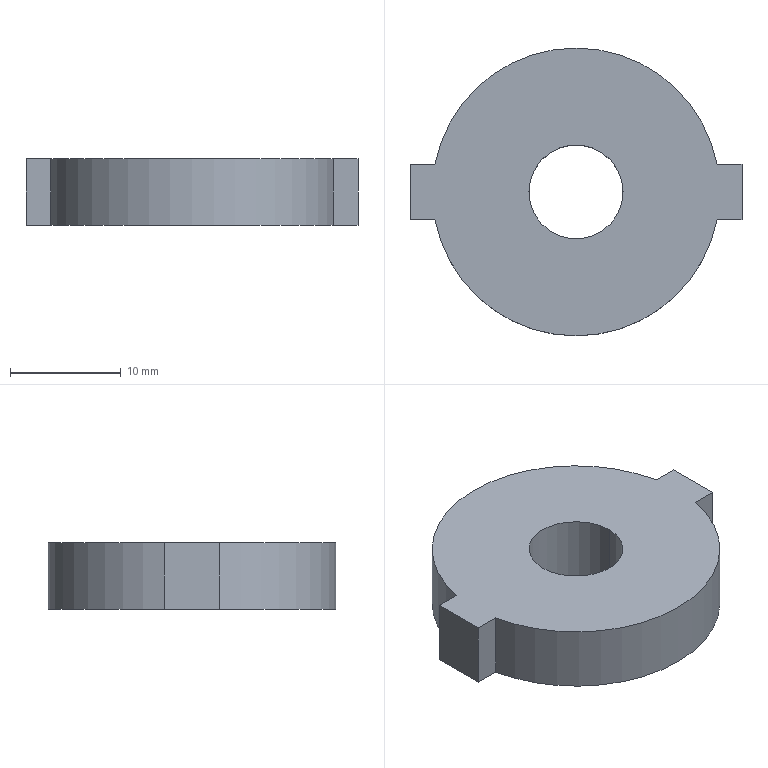Part | SolidWorks | features Extrusion 1 | 1 solid | 12 faces | box 30 x 26 x 6 mm | volume 2970 mm3 | plane 8 | cylinder 4 | commonest cylinder face diameters 8.5 x2 26 x2
STEP:
#1=CARTESIAN_POINT('',(-4.25,0.,0.));
#2=VERTEX_POINT('',#1);
#3=CARTESIAN_POINT('',(4.25,0.,0.));
#4=VERTEX_POINT('',#3);
#5=CARTESIAN_POINT('',(0.,0.,0.));
#6=DIRECTION('',(0.,0.,1.));
#7=DIRECTION('',(-1.,0.,0.));
#8=AXIS2_PLACEMENT_3D('',#5,#6,#7);
#9=CIRCLE('',#8,4.25);
#10=EDGE_CURVE('',#2,#4,#9,.T.);
#11=ORIENTED_EDGE('',*,*,#10,.F.);
#12=CARTESIAN_POINT('',(-4.25,0.,6.));
#13=VERTEX_POINT('',#12);
#14=CARTESIAN_POINT('',(-4.25,0.,0.));
#15=DIRECTION('',(0.,0.,1.));
#16=VECTOR('',#15,1000.);
#17=LINE('',#14,#16);
#18=EDGE_CURVE('',#2,#13,#17,.T.);
#19=ORIENTED_EDGE('',*,*,#18,.T.);
#20=CARTESIAN_POINT('',(4.25,0.,6.));
#21=VERTEX_POINT('',#20);
#22=CARTESIAN_POINT('',(0.,0.,6.));
#23=DIRECTION('',(0.,0.,1.));
#24=DIRECTION('',(-1.,0.,0.));
#25=AXIS2_PLACEMENT_3D('',#22,#23,#24);
#26=CIRCLE('',#25,4.25);
#27=EDGE_CURVE('',#13,#21,#26,.T.);
#28=ORIENTED_EDGE('',*,*,#27,.T.);
#29=CARTESIAN_POINT('',(4.25,0.,0.));
#30=DIRECTION('',(0.,0.,1.));
#31=VECTOR('',#30,1000.);
#32=LINE('',#29,#31);
#33=EDGE_CURVE('',#4,#21,#32,.T.);
#34=ORIENTED_EDGE('',*,*,#33,.F.);
#35=EDGE_LOOP('',(#11,#19,#28,#34));
#36=FACE_OUTER_BOUND('',#35,.T.);
#37=CARTESIAN_POINT('',(0.,0.,0.));
#38=DIRECTION('',(0.,0.,1.));
#39=DIRECTION('',(1.,0.,0.));
#40=AXIS2_PLACEMENT_3D('',#37,#38,#39);
#41=CYLINDRICAL_SURFACE('',#40,4.25);
#42=ADVANCED_FACE('',(#36),#41,.F.);
#43=CARTESIAN_POINT('',(12.757,2.5,6.));
#44=VERTEX_POINT('',#43);
#45=CARTESIAN_POINT('',(-12.757,2.5,6.));
#46=VERTEX_POINT('',#45);
#47=CARTESIAN_POINT('',(0.,0.,6.));
#48=DIRECTION('',(0.,0.,1.));
#49=DIRECTION('',(1.,0.,0.));
#50=AXIS2_PLACEMENT_3D('',#47,#48,#49);
#51=CIRCLE('',#50,13.);
#52=EDGE_CURVE('',#44,#46,#51,.T.);
#53=ORIENTED_EDGE('',*,*,#52,.F.);
#54=CARTESIAN_POINT('',(12.757,2.5,0.));
#55=VERTEX_POINT('',#54);
#56=CARTESIAN_POINT('',(12.757,2.5,0.));
#57=DIRECTION('',(0.,0.,1.));
#58=VECTOR('',#57,1000.);
#59=LINE('',#56,#58);
#60=EDGE_CURVE('',#55,#44,#59,.T.);
#61=ORIENTED_EDGE('',*,*,#60,.F.);
#62=CARTESIAN_POINT('',(-12.757,2.5,0.));
#63=VERTEX_POINT('',#62);
#64=CARTESIAN_POINT('',(0.,0.,0.));
#65=DIRECTION('',(0.,0.,1.));
#66=DIRECTION('',(1.,0.,0.));
#67=AXIS2_PLACEMENT_3D('',#64,#65,#66);
#68=CIRCLE('',#67,13.);
#69=EDGE_CURVE('',#55,#63,#68,.T.);
#70=ORIENTED_EDGE('',*,*,#69,.T.);
#71=CARTESIAN_POINT('',(-12.757,2.5,0.));
#72=DIRECTION('',(0.,0.,1.));
#73=VECTOR('',#72,1000.);
#74=LINE('',#71,#73);
#75=EDGE_CURVE('',#63,#46,#74,.T.);
#76=ORIENTED_EDGE('',*,*,#75,.T.);
#77=EDGE_LOOP('',(#53,#61,#70,#76));
#78=FACE_OUTER_BOUND('',#77,.T.);
#79=CARTESIAN_POINT('',(0.,0.,0.));
#80=DIRECTION('',(0.,0.,1.));
#81=DIRECTION('',(1.,0.,0.));
#82=AXIS2_PLACEMENT_3D('',#79,#80,#81);
#83=CYLINDRICAL_SURFACE('',#82,13.);
#84=ADVANCED_FACE('',(#78),#83,.T.);
#85=CARTESIAN_POINT('',(15.,2.5,6.));
#86=VERTEX_POINT('',#85);
#87=CARTESIAN_POINT('',(15.,2.5,6.));
#88=DIRECTION('',(-1.,0.,0.));
#89=VECTOR('',#88,1000.);
#90=LINE('',#87,#89);
#91=EDGE_CURVE('',#86,#44,#90,.T.);
#92=ORIENTED_EDGE('',*,*,#91,.F.);
#93=CARTESIAN_POINT('',(15.,2.5,0.));
#94=VERTEX_POINT('',#93);
#95=CARTESIAN_POINT('',(15.,2.5,0.));
#96=DIRECTION('',(0.,0.,1.));
#97=VECTOR('',#96,1000.);
#98=LINE('',#95,#97);
#99=EDGE_CURVE('',#94,#86,#98,.T.);
#100=ORIENTED_EDGE('',*,*,#99,.F.);
#101=CARTESIAN_POINT('',(15.,2.5,0.));
#102=DIRECTION('',(-1.,0.,0.));
#103=VECTOR('',#102,1000.);
#104=LINE('',#101,#103);
#105=EDGE_CURVE('',#94,#55,#104,.T.);
#106=ORIENTED_EDGE('',*,*,#105,.T.);
#107=ORIENTED_EDGE('',*,*,#60,.T.);
#108=EDGE_LOOP('',(#92,#100,#106,#107));
#109=FACE_OUTER_BOUND('',#108,.T.);
#110=CARTESIAN_POINT('',(15.,2.5,0.));
#111=DIRECTION('',(0.,1.,0.));
#112=DIRECTION('',(0.,0.,1.));
#113=AXIS2_PLACEMENT_3D('',#110,#111,#112);
#114=PLANE('',#113);
#115=ADVANCED_FACE('',(#109),#114,.T.);
#116=CARTESIAN_POINT('',(15.,-2.5,6.));
#117=VERTEX_POINT('',#116);
#118=CARTESIAN_POINT('',(15.,-2.5,6.));
#119=DIRECTION('',(0.,1.,0.));
#120=VECTOR('',#119,1000.);
#121=LINE('',#118,#120);
#122=EDGE_CURVE('',#117,#86,#121,.T.);
#123=ORIENTED_EDGE('',*,*,#122,.F.);
#124=CARTESIAN_POINT('',(15.,-2.5,0.));
#125=VERTEX_POINT('',#124);
#126=CARTESIAN_POINT('',(15.,-2.5,0.));
#127=DIRECTION('',(0.,0.,1.));
#128=VECTOR('',#127,1000.);
#129=LINE('',#126,#128);
#130=EDGE_CURVE('',#125,#117,#129,.T.);
#131=ORIENTED_EDGE('',*,*,#130,.F.);
#132=CARTESIAN_POINT('',(15.,-2.5,0.));
#133=DIRECTION('',(0.,1.,0.));
#134=VECTOR('',#133,1000.);
#135=LINE('',#132,#134);
#136=EDGE_CURVE('',#125,#94,#135,.T.);
#137=ORIENTED_EDGE('',*,*,#136,.T.);
#138=ORIENTED_EDGE('',*,*,#99,.T.);
#139=EDGE_LOOP('',(#123,#131,#137,#138));
#140=FACE_OUTER_BOUND('',#139,.T.);
#141=CARTESIAN_POINT('',(15.,-2.5,0.));
#142=DIRECTION('',(1.,0.,0.));
#143=DIRECTION('',(0.,0.,-1.));
#144=AXIS2_PLACEMENT_3D('',#141,#142,#143);
#145=PLANE('',#144);
#146=ADVANCED_FACE('',(#140),#145,.T.);
#147=CARTESIAN_POINT('',(12.757,-2.5,6.));
#148=VERTEX_POINT('',#147);
#149=CARTESIAN_POINT('',(12.757,-2.5,6.));
#150=DIRECTION('',(1.,0.,0.));
#151=VECTOR('',#150,1000.);
#152=LINE('',#149,#151);
#153=EDGE_CURVE('',#148,#117,#152,.T.);
#154=ORIENTED_EDGE('',*,*,#153,.F.);
#155=CARTESIAN_POINT('',(12.757,-2.5,0.));
#156=VERTEX_POINT('',#155);
#157=CARTESIAN_POINT('',(12.757,-2.5,0.));
#158=DIRECTION('',(0.,0.,1.));
#159=VECTOR('',#158,1000.);
#160=LINE('',#157,#159);
#161=EDGE_CURVE('',#156,#148,#160,.T.);
#162=ORIENTED_EDGE('',*,*,#161,.F.);
#163=CARTESIAN_POINT('',(12.757,-2.5,0.));
#164=DIRECTION('',(1.,0.,0.));
#165=VECTOR('',#164,1000.);
#166=LINE('',#163,#165);
#167=EDGE_CURVE('',#156,#125,#166,.T.);
#168=ORIENTED_EDGE('',*,*,#167,.T.);
#169=ORIENTED_EDGE('',*,*,#130,.T.);
#170=EDGE_LOOP('',(#154,#162,#168,#169));
#171=FACE_OUTER_BOUND('',#170,.T.);
#172=CARTESIAN_POINT('',(12.757,-2.5,0.));
#173=DIRECTION('',(0.,-1.,0.));
#174=DIRECTION('',(0.,0.,-1.));
#175=AXIS2_PLACEMENT_3D('',#172,#173,#174);
#176=PLANE('',#175);
#177=ADVANCED_FACE('',(#171),#176,.T.);
#178=CARTESIAN_POINT('',(-12.757,-2.5,6.));
#179=VERTEX_POINT('',#178);
#180=CARTESIAN_POINT('',(0.,0.,6.));
#181=DIRECTION('',(0.,0.,1.));
#182=DIRECTION('',(1.,0.,0.));
#183=AXIS2_PLACEMENT_3D('',#180,#181,#182);
#184=CIRCLE('',#183,13.);
#185=EDGE_CURVE('',#179,#148,#184,.T.);
#186=ORIENTED_EDGE('',*,*,#185,.F.);
#187=CARTESIAN_POINT('',(-12.757,-2.5,0.));
#188=VERTEX_POINT('',#187);
#189=CARTESIAN_POINT('',(-12.757,-2.5,0.));
#190=DIRECTION('',(0.,0.,1.));
#191=VECTOR('',#190,1000.);
#192=LINE('',#189,#191);
#193=EDGE_CURVE('',#188,#179,#192,.T.);
#194=ORIENTED_EDGE('',*,*,#193,.F.);
#195=CARTESIAN_POINT('',(0.,0.,0.));
#196=DIRECTION('',(0.,0.,1.));
#197=DIRECTION('',(1.,0.,0.));
#198=AXIS2_PLACEMENT_3D('',#195,#196,#197);
#199=CIRCLE('',#198,13.);
#200=EDGE_CURVE('',#188,#156,#199,.T.);
#201=ORIENTED_EDGE('',*,*,#200,.T.);
#202=ORIENTED_EDGE('',*,*,#161,.T.);
#203=EDGE_LOOP('',(#186,#194,#201,#202));
#204=FACE_OUTER_BOUND('',#203,.T.);
#205=CARTESIAN_POINT('',(0.,0.,0.));
#206=DIRECTION('',(0.,0.,1.));
#207=DIRECTION('',(1.,0.,0.));
#208=AXIS2_PLACEMENT_3D('',#205,#206,#207);
#209=CYLINDRICAL_SURFACE('',#208,13.);
#210=ADVANCED_FACE('',(#204),#209,.T.);
#211=CARTESIAN_POINT('',(-15.,-2.5,6.));
#212=VERTEX_POINT('',#211);
#213=CARTESIAN_POINT('',(-15.,-2.5,6.));
#214=DIRECTION('',(1.,0.,0.));
#215=VECTOR('',#214,1000.);
#216=LINE('',#213,#215);
#217=EDGE_CURVE('',#212,#179,#216,.T.);
#218=ORIENTED_EDGE('',*,*,#217,.F.);
#219=CARTESIAN_POINT('',(-15.,-2.5,0.));
#220=VERTEX_POINT('',#219);
#221=CARTESIAN_POINT('',(-15.,-2.5,0.));
#222=DIRECTION('',(0.,0.,1.));
#223=VECTOR('',#222,1000.);
#224=LINE('',#221,#223);
#225=EDGE_CURVE('',#220,#212,#224,.T.);
#226=ORIENTED_EDGE('',*,*,#225,.F.);
#227=CARTESIAN_POINT('',(-15.,-2.5,0.));
#228=DIRECTION('',(1.,0.,0.));
#229=VECTOR('',#228,1000.);
#230=LINE('',#227,#229);
#231=EDGE_CURVE('',#220,#188,#230,.T.);
#232=ORIENTED_EDGE('',*,*,#231,.T.);
#233=ORIENTED_EDGE('',*,*,#193,.T.);
#234=EDGE_LOOP('',(#218,#226,#232,#233));
#235=FACE_OUTER_BOUND('',#234,.T.);
#236=CARTESIAN_POINT('',(-15.,-2.5,0.));
#237=DIRECTION('',(0.,-1.,0.));
#238=DIRECTION('',(0.,0.,-1.));
#239=AXIS2_PLACEMENT_3D('',#236,#237,#238);
#240=PLANE('',#239);
#241=ADVANCED_FACE('',(#235),#240,.T.);
#242=CARTESIAN_POINT('',(-15.,2.5,6.));
#243=VERTEX_POINT('',#242);
#244=CARTESIAN_POINT('',(-15.,2.5,6.));
#245=DIRECTION('',(0.,-1.,0.));
#246=VECTOR('',#245,1000.);
#247=LINE('',#244,#246);
#248=EDGE_CURVE('',#243,#212,#247,.T.);
#249=ORIENTED_EDGE('',*,*,#248,.F.);
#250=CARTESIAN_POINT('',(-15.,2.5,0.));
#251=VERTEX_POINT('',#250);
#252=CARTESIAN_POINT('',(-15.,2.5,0.));
#253=DIRECTION('',(0.,0.,1.));
#254=VECTOR('',#253,1000.);
#255=LINE('',#252,#254);
#256=EDGE_CURVE('',#251,#243,#255,.T.);
#257=ORIENTED_EDGE('',*,*,#256,.F.);
#258=CARTESIAN_POINT('',(-15.,2.5,0.));
#259=DIRECTION('',(0.,-1.,0.));
#260=VECTOR('',#259,1000.);
#261=LINE('',#258,#260);
#262=EDGE_CURVE('',#251,#220,#261,.T.);
#263=ORIENTED_EDGE('',*,*,#262,.T.);
#264=ORIENTED_EDGE('',*,*,#225,.T.);
#265=EDGE_LOOP('',(#249,#257,#263,#264));
#266=FACE_OUTER_BOUND('',#265,.T.);
#267=CARTESIAN_POINT('',(-15.,2.5,0.));
#268=DIRECTION('',(-1.,0.,0.));
#269=DIRECTION('',(0.,0.,1.));
#270=AXIS2_PLACEMENT_3D('',#267,#268,#269);
#271=PLANE('',#270);
#272=ADVANCED_FACE('',(#266),#271,.T.);
#273=CARTESIAN_POINT('',(-12.757,2.5,6.));
#274=DIRECTION('',(-1.,0.,0.));
#275=VECTOR('',#274,1000.);
#276=LINE('',#273,#275);
#277=EDGE_CURVE('',#46,#243,#276,.T.);
#278=ORIENTED_EDGE('',*,*,#277,.F.);
#279=ORIENTED_EDGE('',*,*,#75,.F.);
#280=CARTESIAN_POINT('',(-12.757,2.5,0.));
#281=DIRECTION('',(-1.,0.,0.));
#282=VECTOR('',#281,1000.);
#283=LINE('',#280,#282);
#284=EDGE_CURVE('',#63,#251,#283,.T.);
#285=ORIENTED_EDGE('',*,*,#284,.T.);
#286=ORIENTED_EDGE('',*,*,#256,.T.);
#287=EDGE_LOOP('',(#278,#279,#285,#286));
#288=FACE_OUTER_BOUND('',#287,.T.);
#289=CARTESIAN_POINT('',(-12.757,2.5,0.));
#290=DIRECTION('',(0.,1.,0.));
#291=DIRECTION('',(0.,0.,1.));
#292=AXIS2_PLACEMENT_3D('',#289,#290,#291);
#293=PLANE('',#292);
#294=ADVANCED_FACE('',(#288),#293,.T.);
#295=CARTESIAN_POINT('',(0.,0.,0.));
#296=DIRECTION('',(0.,0.,1.));
#297=DIRECTION('',(-1.,0.,0.));
#298=AXIS2_PLACEMENT_3D('',#295,#296,#297);
#299=CIRCLE('',#298,4.25);
#300=EDGE_CURVE('',#4,#2,#299,.T.);
#301=ORIENTED_EDGE('',*,*,#300,.T.);
#302=ORIENTED_EDGE('',*,*,#10,.T.);
#303=EDGE_LOOP('',(#301,#302));
#304=FACE_BOUND('',#303,.T.);
#305=ORIENTED_EDGE('',*,*,#69,.F.);
#306=ORIENTED_EDGE('',*,*,#105,.F.);
#307=ORIENTED_EDGE('',*,*,#136,.F.);
#308=ORIENTED_EDGE('',*,*,#167,.F.);
#309=ORIENTED_EDGE('',*,*,#200,.F.);
#310=ORIENTED_EDGE('',*,*,#231,.F.);
#311=ORIENTED_EDGE('',*,*,#262,.F.);
#312=ORIENTED_EDGE('',*,*,#284,.F.);
#313=EDGE_LOOP('',(#305,#306,#307,#308,#309,#310,#311,#312));
#314=FACE_OUTER_BOUND('',#313,.T.);
#315=CARTESIAN_POINT('',(0.,0.,0.));
#316=DIRECTION('',(0.,0.,1.));
#317=DIRECTION('',(1.,0.,0.));
#318=AXIS2_PLACEMENT_3D('',#315,#316,#317);
#319=PLANE('',#318);
#320=ADVANCED_FACE('',(#304,#314),#319,.F.);
#321=CARTESIAN_POINT('',(0.,0.,6.));
#322=DIRECTION('',(0.,0.,1.));
#323=DIRECTION('',(-1.,0.,0.));
#324=AXIS2_PLACEMENT_3D('',#321,#322,#323);
#325=CIRCLE('',#324,4.25);
#326=EDGE_CURVE('',#21,#13,#325,.T.);
#327=ORIENTED_EDGE('',*,*,#326,.F.);
#328=ORIENTED_EDGE('',*,*,#27,.F.);
#329=EDGE_LOOP('',(#327,#328));
#330=FACE_BOUND('',#329,.T.);
#331=ORIENTED_EDGE('',*,*,#52,.T.);
#332=ORIENTED_EDGE('',*,*,#277,.T.);
#333=ORIENTED_EDGE('',*,*,#248,.T.);
#334=ORIENTED_EDGE('',*,*,#217,.T.);
#335=ORIENTED_EDGE('',*,*,#185,.T.);
#336=ORIENTED_EDGE('',*,*,#153,.T.);
#337=ORIENTED_EDGE('',*,*,#122,.T.);
#338=ORIENTED_EDGE('',*,*,#91,.T.);
#339=EDGE_LOOP('',(#331,#332,#333,#334,#335,#336,#337,#338));
#340=FACE_OUTER_BOUND('',#339,.T.);
#341=CARTESIAN_POINT('',(0.,0.,6.));
#342=DIRECTION('',(0.,0.,1.));
#343=DIRECTION('',(1.,0.,0.));
#344=AXIS2_PLACEMENT_3D('',#341,#342,#343);
#345=PLANE('',#344);
#346=ADVANCED_FACE('',(#330,#340),#345,.T.);
#347=ORIENTED_EDGE('',*,*,#18,.F.);
#348=ORIENTED_EDGE('',*,*,#300,.F.);
#349=ORIENTED_EDGE('',*,*,#33,.T.);
#350=ORIENTED_EDGE('',*,*,#326,.T.);
#351=EDGE_LOOP('',(#347,#348,#349,#350));
#352=FACE_OUTER_BOUND('',#351,.T.);
#353=CARTESIAN_POINT('',(0.,0.,0.));
#354=DIRECTION('',(0.,0.,1.));
#355=DIRECTION('',(1.,0.,0.));
#356=AXIS2_PLACEMENT_3D('',#353,#354,#355);
#357=CYLINDRICAL_SURFACE('',#356,4.25);
#358=ADVANCED_FACE('',(#352),#357,.F.);
#359=CLOSED_SHELL('',(#42,#84,#115,#146,#177,#210,#241,#272,#294,#320,#346,#358));
#360=MANIFOLD_SOLID_BREP('',#359);
#361=CARTESIAN_POINT('',(0.,0.,0.));
#362=DIRECTION('',(0.,0.,1.));
#363=DIRECTION('',(1.,0.,0.));
#364=AXIS2_PLACEMENT_3D('',#361,#362,#363);
#365=(LENGTH_UNIT()NAMED_UNIT(*)SI_UNIT(.MILLI.,.METRE.));
#366=UNCERTAINTY_MEASURE_WITH_UNIT(LENGTH_MEASURE(0.00001),#365,'','');
#367=(NAMED_UNIT(*)PLANE_ANGLE_UNIT()SI_UNIT($,.RADIAN.));
#368=(NAMED_UNIT(*)SI_UNIT($,.STERADIAN.)SOLID_ANGLE_UNIT());
#369=(GEOMETRIC_REPRESENTATION_CONTEXT(3)GLOBAL_UNCERTAINTY_ASSIGNED_CONTEXT((#366))GLOBAL_UNIT_ASSIGNED_CONTEXT((#365,#367,#368))REPRESENTATION_CONTEXT('',''));
#370=ADVANCED_BREP_SHAPE_REPRESENTATION('',(#360,#364),#369);